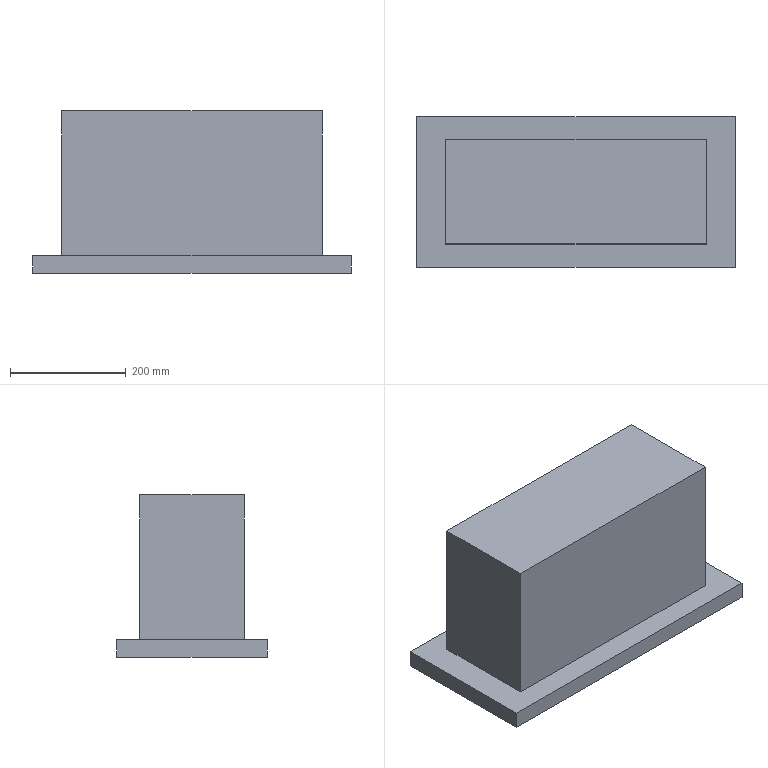Part | SolidWorks | features Extrusion 1, ICE 1 | 1 solid | 11 faces | box 550 x 260 x 280 mm | volume 24540000 mm3 | plane 11
STEP:
#1=CARTESIAN_POINT('',(0.,180.,30.));
#2=VERTEX_POINT('',#1);
#3=CARTESIAN_POINT('',(0.,180.,280.));
#4=VERTEX_POINT('',#3);
#5=CARTESIAN_POINT('',(0.,180.,280.));
#6=DIRECTION('',(0.,0.,1.));
#7=VECTOR('',#6,1000.);
#8=LINE('',#5,#7);
#9=EDGE_CURVE('',#2,#4,#8,.T.);
#10=ORIENTED_EDGE('',*,*,#9,.F.);
#11=CARTESIAN_POINT('',(0.,0.,30.));
#12=VERTEX_POINT('',#11);
#13=CARTESIAN_POINT('',(0.,180.,30.));
#14=DIRECTION('',(0.,-1.,0.));
#15=VECTOR('',#14,1000.);
#16=LINE('',#13,#15);
#17=EDGE_CURVE('',#2,#12,#16,.T.);
#18=ORIENTED_EDGE('',*,*,#17,.T.);
#19=CARTESIAN_POINT('',(0.,0.,280.));
#20=VERTEX_POINT('',#19);
#21=CARTESIAN_POINT('',(0.,0.,280.));
#22=DIRECTION('',(0.,0.,1.));
#23=VECTOR('',#22,1000.);
#24=LINE('',#21,#23);
#25=EDGE_CURVE('',#12,#20,#24,.T.);
#26=ORIENTED_EDGE('',*,*,#25,.T.);
#27=CARTESIAN_POINT('',(0.,180.,280.));
#28=DIRECTION('',(0.,-1.,0.));
#29=VECTOR('',#28,1000.);
#30=LINE('',#27,#29);
#31=EDGE_CURVE('',#4,#20,#30,.T.);
#32=ORIENTED_EDGE('',*,*,#31,.F.);
#33=EDGE_LOOP('',(#10,#18,#26,#32));
#34=FACE_OUTER_BOUND('',#33,.T.);
#35=CARTESIAN_POINT('',(0.,180.,280.));
#36=DIRECTION('',(1.,0.,0.));
#37=DIRECTION('',(0.,0.,-1.));
#38=AXIS2_PLACEMENT_3D('',#35,#36,#37);
#39=PLANE('',#38);
#40=ADVANCED_FACE('',(#34),#39,.F.);
#41=CARTESIAN_POINT('',(450.,0.,280.));
#42=VERTEX_POINT('',#41);
#43=CARTESIAN_POINT('',(450.,0.,280.));
#44=DIRECTION('',(1.,0.,0.));
#45=VECTOR('',#44,1000.);
#46=LINE('',#43,#45);
#47=EDGE_CURVE('',#20,#42,#46,.T.);
#48=ORIENTED_EDGE('',*,*,#47,.T.);
#49=CARTESIAN_POINT('',(450.,180.,280.));
#50=VERTEX_POINT('',#49);
#51=CARTESIAN_POINT('',(450.,180.,280.));
#52=DIRECTION('',(0.,-1.,0.));
#53=VECTOR('',#52,1000.);
#54=LINE('',#51,#53);
#55=EDGE_CURVE('',#50,#42,#54,.T.);
#56=ORIENTED_EDGE('',*,*,#55,.F.);
#57=CARTESIAN_POINT('',(450.,180.,280.));
#58=DIRECTION('',(1.,0.,0.));
#59=VECTOR('',#58,1000.);
#60=LINE('',#57,#59);
#61=EDGE_CURVE('',#4,#50,#60,.T.);
#62=ORIENTED_EDGE('',*,*,#61,.F.);
#63=ORIENTED_EDGE('',*,*,#31,.T.);
#64=EDGE_LOOP('',(#48,#56,#62,#63));
#65=FACE_OUTER_BOUND('',#64,.T.);
#66=CARTESIAN_POINT('',(450.,180.,280.));
#67=DIRECTION('',(0.,0.,-1.));
#68=DIRECTION('',(-1.,0.,0.));
#69=AXIS2_PLACEMENT_3D('',#66,#67,#68);
#70=PLANE('',#69);
#71=ADVANCED_FACE('',(#65),#70,.F.);
#72=CARTESIAN_POINT('',(450.,0.,30.));
#73=VERTEX_POINT('',#72);
#74=CARTESIAN_POINT('',(450.,0.,0.));
#75=DIRECTION('',(0.,0.,-1.));
#76=VECTOR('',#75,1000.);
#77=LINE('',#74,#76);
#78=EDGE_CURVE('',#42,#73,#77,.T.);
#79=ORIENTED_EDGE('',*,*,#78,.T.);
#80=CARTESIAN_POINT('',(450.,180.,30.));
#81=VERTEX_POINT('',#80);
#82=CARTESIAN_POINT('',(450.,180.,30.));
#83=DIRECTION('',(0.,1.,0.));
#84=VECTOR('',#83,1000.);
#85=LINE('',#82,#84);
#86=EDGE_CURVE('',#73,#81,#85,.T.);
#87=ORIENTED_EDGE('',*,*,#86,.T.);
#88=CARTESIAN_POINT('',(450.,180.,0.));
#89=DIRECTION('',(0.,0.,-1.));
#90=VECTOR('',#89,1000.);
#91=LINE('',#88,#90);
#92=EDGE_CURVE('',#50,#81,#91,.T.);
#93=ORIENTED_EDGE('',*,*,#92,.F.);
#94=ORIENTED_EDGE('',*,*,#55,.T.);
#95=EDGE_LOOP('',(#79,#87,#93,#94));
#96=FACE_OUTER_BOUND('',#95,.T.);
#97=CARTESIAN_POINT('',(450.,180.,0.));
#98=DIRECTION('',(-1.,0.,0.));
#99=DIRECTION('',(0.,0.,1.));
#100=AXIS2_PLACEMENT_3D('',#97,#98,#99);
#101=PLANE('',#100);
#102=ADVANCED_FACE('',(#96),#101,.F.);
#103=ORIENTED_EDGE('',*,*,#92,.T.);
#104=CARTESIAN_POINT('',(0.,180.,30.));
#105=DIRECTION('',(-1.,0.,0.));
#106=VECTOR('',#105,1000.);
#107=LINE('',#104,#106);
#108=EDGE_CURVE('',#81,#2,#107,.T.);
#109=ORIENTED_EDGE('',*,*,#108,.T.);
#110=ORIENTED_EDGE('',*,*,#9,.T.);
#111=ORIENTED_EDGE('',*,*,#61,.T.);
#112=EDGE_LOOP('',(#103,#109,#110,#111));
#113=FACE_OUTER_BOUND('',#112,.T.);
#114=CARTESIAN_POINT('',(0.,180.,0.));
#115=DIRECTION('',(0.,-1.,0.));
#116=DIRECTION('',(0.,0.,-1.));
#117=AXIS2_PLACEMENT_3D('',#114,#115,#116);
#118=PLANE('',#117);
#119=ADVANCED_FACE('',(#113),#118,.F.);
#120=CARTESIAN_POINT('',(0.,0.,30.));
#121=DIRECTION('',(-1.,0.,0.));
#122=VECTOR('',#121,1000.);
#123=LINE('',#120,#122);
#124=EDGE_CURVE('',#73,#12,#123,.T.);
#125=ORIENTED_EDGE('',*,*,#124,.F.);
#126=ORIENTED_EDGE('',*,*,#78,.F.);
#127=ORIENTED_EDGE('',*,*,#47,.F.);
#128=ORIENTED_EDGE('',*,*,#25,.F.);
#129=EDGE_LOOP('',(#125,#126,#127,#128));
#130=FACE_OUTER_BOUND('',#129,.T.);
#131=CARTESIAN_POINT('',(0.,0.,0.));
#132=DIRECTION('',(0.,-1.,0.));
#133=DIRECTION('',(0.,0.,-1.));
#134=AXIS2_PLACEMENT_3D('',#131,#132,#133);
#135=PLANE('',#134);
#136=ADVANCED_FACE('',(#130),#135,.T.);
#137=CARTESIAN_POINT('',(-50.,220.,30.));
#138=VERTEX_POINT('',#137);
#139=CARTESIAN_POINT('',(-50.,-40.,30.));
#140=VERTEX_POINT('',#139);
#141=CARTESIAN_POINT('',(-50.,220.,30.));
#142=DIRECTION('',(0.,-1.,0.));
#143=VECTOR('',#142,1000.);
#144=LINE('',#141,#143);
#145=EDGE_CURVE('',#138,#140,#144,.T.);
#146=ORIENTED_EDGE('',*,*,#145,.T.);
#147=CARTESIAN_POINT('',(500.,-40.,30.));
#148=VERTEX_POINT('',#147);
#149=CARTESIAN_POINT('',(-50.,-40.,30.));
#150=DIRECTION('',(-1.,0.,0.));
#151=VECTOR('',#150,1000.);
#152=LINE('',#149,#151);
#153=EDGE_CURVE('',#148,#140,#152,.T.);
#154=ORIENTED_EDGE('',*,*,#153,.F.);
#155=CARTESIAN_POINT('',(500.,220.,30.));
#156=VERTEX_POINT('',#155);
#157=CARTESIAN_POINT('',(500.,220.,30.));
#158=DIRECTION('',(0.,-1.,0.));
#159=VECTOR('',#158,1000.);
#160=LINE('',#157,#159);
#161=EDGE_CURVE('',#156,#148,#160,.T.);
#162=ORIENTED_EDGE('',*,*,#161,.F.);
#163=CARTESIAN_POINT('',(-50.,220.,30.));
#164=DIRECTION('',(-1.,0.,0.));
#165=VECTOR('',#164,1000.);
#166=LINE('',#163,#165);
#167=EDGE_CURVE('',#156,#138,#166,.T.);
#168=ORIENTED_EDGE('',*,*,#167,.T.);
#169=EDGE_LOOP('',(#146,#154,#162,#168));
#170=FACE_OUTER_BOUND('',#169,.T.);
#171=ORIENTED_EDGE('',*,*,#108,.F.);
#172=ORIENTED_EDGE('',*,*,#86,.F.);
#173=ORIENTED_EDGE('',*,*,#124,.T.);
#174=ORIENTED_EDGE('',*,*,#17,.F.);
#175=EDGE_LOOP('',(#171,#172,#173,#174));
#176=FACE_BOUND('',#175,.T.);
#177=CARTESIAN_POINT('',(-50.,220.,30.));
#178=DIRECTION('',(0.,0.,1.));
#179=DIRECTION('',(1.,0.,0.));
#180=AXIS2_PLACEMENT_3D('',#177,#178,#179);
#181=PLANE('',#180);
#182=ADVANCED_FACE('',(#170,#176),#181,.T.);
#183=CARTESIAN_POINT('',(-50.,220.,0.));
#184=VERTEX_POINT('',#183);
#185=CARTESIAN_POINT('',(-50.,-40.,0.));
#186=VERTEX_POINT('',#185);
#187=CARTESIAN_POINT('',(-50.,220.,0.));
#188=DIRECTION('',(0.,-1.,0.));
#189=VECTOR('',#188,1000.);
#190=LINE('',#187,#189);
#191=EDGE_CURVE('',#184,#186,#190,.T.);
#192=ORIENTED_EDGE('',*,*,#191,.T.);
#193=CARTESIAN_POINT('',(-50.,-40.,30.));
#194=DIRECTION('',(0.,0.,-1.));
#195=VECTOR('',#194,1000.);
#196=LINE('',#193,#195);
#197=EDGE_CURVE('',#140,#186,#196,.T.);
#198=ORIENTED_EDGE('',*,*,#197,.F.);
#199=ORIENTED_EDGE('',*,*,#145,.F.);
#200=CARTESIAN_POINT('',(-50.,220.,30.));
#201=DIRECTION('',(0.,0.,-1.));
#202=VECTOR('',#201,1000.);
#203=LINE('',#200,#202);
#204=EDGE_CURVE('',#138,#184,#203,.T.);
#205=ORIENTED_EDGE('',*,*,#204,.T.);
#206=EDGE_LOOP('',(#192,#198,#199,#205));
#207=FACE_OUTER_BOUND('',#206,.T.);
#208=CARTESIAN_POINT('',(-50.,220.,30.));
#209=DIRECTION('',(-1.,0.,0.));
#210=DIRECTION('',(0.,0.,1.));
#211=AXIS2_PLACEMENT_3D('',#208,#209,#210);
#212=PLANE('',#211);
#213=ADVANCED_FACE('',(#207),#212,.T.);
#214=ORIENTED_EDGE('',*,*,#161,.T.);
#215=CARTESIAN_POINT('',(500.,-40.,0.));
#216=VERTEX_POINT('',#215);
#217=CARTESIAN_POINT('',(500.,-40.,30.));
#218=DIRECTION('',(0.,0.,1.));
#219=VECTOR('',#218,1000.);
#220=LINE('',#217,#219);
#221=EDGE_CURVE('',#216,#148,#220,.T.);
#222=ORIENTED_EDGE('',*,*,#221,.F.);
#223=CARTESIAN_POINT('',(500.,220.,0.));
#224=VERTEX_POINT('',#223);
#225=CARTESIAN_POINT('',(500.,220.,0.));
#226=DIRECTION('',(0.,-1.,0.));
#227=VECTOR('',#226,1000.);
#228=LINE('',#225,#227);
#229=EDGE_CURVE('',#224,#216,#228,.T.);
#230=ORIENTED_EDGE('',*,*,#229,.F.);
#231=CARTESIAN_POINT('',(500.,220.,30.));
#232=DIRECTION('',(0.,0.,1.));
#233=VECTOR('',#232,1000.);
#234=LINE('',#231,#233);
#235=EDGE_CURVE('',#224,#156,#234,.T.);
#236=ORIENTED_EDGE('',*,*,#235,.T.);
#237=EDGE_LOOP('',(#214,#222,#230,#236));
#238=FACE_OUTER_BOUND('',#237,.T.);
#239=CARTESIAN_POINT('',(500.,220.,30.));
#240=DIRECTION('',(1.,0.,0.));
#241=DIRECTION('',(0.,0.,-1.));
#242=AXIS2_PLACEMENT_3D('',#239,#240,#241);
#243=PLANE('',#242);
#244=ADVANCED_FACE('',(#238),#243,.T.);
#245=ORIENTED_EDGE('',*,*,#204,.F.);
#246=ORIENTED_EDGE('',*,*,#167,.F.);
#247=ORIENTED_EDGE('',*,*,#235,.F.);
#248=CARTESIAN_POINT('',(-50.,220.,0.));
#249=DIRECTION('',(1.,0.,0.));
#250=VECTOR('',#249,1000.);
#251=LINE('',#248,#250);
#252=EDGE_CURVE('',#184,#224,#251,.T.);
#253=ORIENTED_EDGE('',*,*,#252,.F.);
#254=EDGE_LOOP('',(#245,#246,#247,#253));
#255=FACE_OUTER_BOUND('',#254,.T.);
#256=CARTESIAN_POINT('',(0.,220.,0.));
#257=DIRECTION('',(0.,-1.,0.));
#258=DIRECTION('',(0.,0.,-1.));
#259=AXIS2_PLACEMENT_3D('',#256,#257,#258);
#260=PLANE('',#259);
#261=ADVANCED_FACE('',(#255),#260,.F.);
#262=ORIENTED_EDGE('',*,*,#197,.T.);
#263=CARTESIAN_POINT('',(-50.,-40.,0.));
#264=DIRECTION('',(1.,0.,0.));
#265=VECTOR('',#264,1000.);
#266=LINE('',#263,#265);
#267=EDGE_CURVE('',#186,#216,#266,.T.);
#268=ORIENTED_EDGE('',*,*,#267,.T.);
#269=ORIENTED_EDGE('',*,*,#221,.T.);
#270=ORIENTED_EDGE('',*,*,#153,.T.);
#271=EDGE_LOOP('',(#262,#268,#269,#270));
#272=FACE_OUTER_BOUND('',#271,.T.);
#273=CARTESIAN_POINT('',(0.,-40.,0.));
#274=DIRECTION('',(0.,-1.,0.));
#275=DIRECTION('',(0.,0.,-1.));
#276=AXIS2_PLACEMENT_3D('',#273,#274,#275);
#277=PLANE('',#276);
#278=ADVANCED_FACE('',(#272),#277,.T.);
#279=ORIENTED_EDGE('',*,*,#229,.T.);
#280=ORIENTED_EDGE('',*,*,#267,.F.);
#281=ORIENTED_EDGE('',*,*,#191,.F.);
#282=ORIENTED_EDGE('',*,*,#252,.T.);
#283=EDGE_LOOP('',(#279,#280,#281,#282));
#284=FACE_OUTER_BOUND('',#283,.T.);
#285=CARTESIAN_POINT('',(0.,180.,0.));
#286=DIRECTION('',(0.,0.,1.));
#287=DIRECTION('',(1.,0.,0.));
#288=AXIS2_PLACEMENT_3D('',#285,#286,#287);
#289=PLANE('',#288);
#290=ADVANCED_FACE('',(#284),#289,.F.);
#291=CLOSED_SHELL('',(#40,#71,#102,#119,#136,#182,#213,#244,#261,#278,#290));
#292=MANIFOLD_SOLID_BREP('',#291);
#293=CARTESIAN_POINT('',(0.,0.,0.));
#294=DIRECTION('',(0.,0.,1.));
#295=DIRECTION('',(1.,0.,0.));
#296=AXIS2_PLACEMENT_3D('',#293,#294,#295);
#297=(LENGTH_UNIT()NAMED_UNIT(*)SI_UNIT(.MILLI.,.METRE.));
#298=UNCERTAINTY_MEASURE_WITH_UNIT(LENGTH_MEASURE(0.00001),#297,'','');
#299=(NAMED_UNIT(*)PLANE_ANGLE_UNIT()SI_UNIT($,.RADIAN.));
#300=(NAMED_UNIT(*)SI_UNIT($,.STERADIAN.)SOLID_ANGLE_UNIT());
#301=(GEOMETRIC_REPRESENTATION_CONTEXT(3)GLOBAL_UNCERTAINTY_ASSIGNED_CONTEXT((#298))GLOBAL_UNIT_ASSIGNED_CONTEXT((#297,#299,#300))REPRESENTATION_CONTEXT('',''));
#302=ADVANCED_BREP_SHAPE_REPRESENTATION('',(#292,#296),#301);